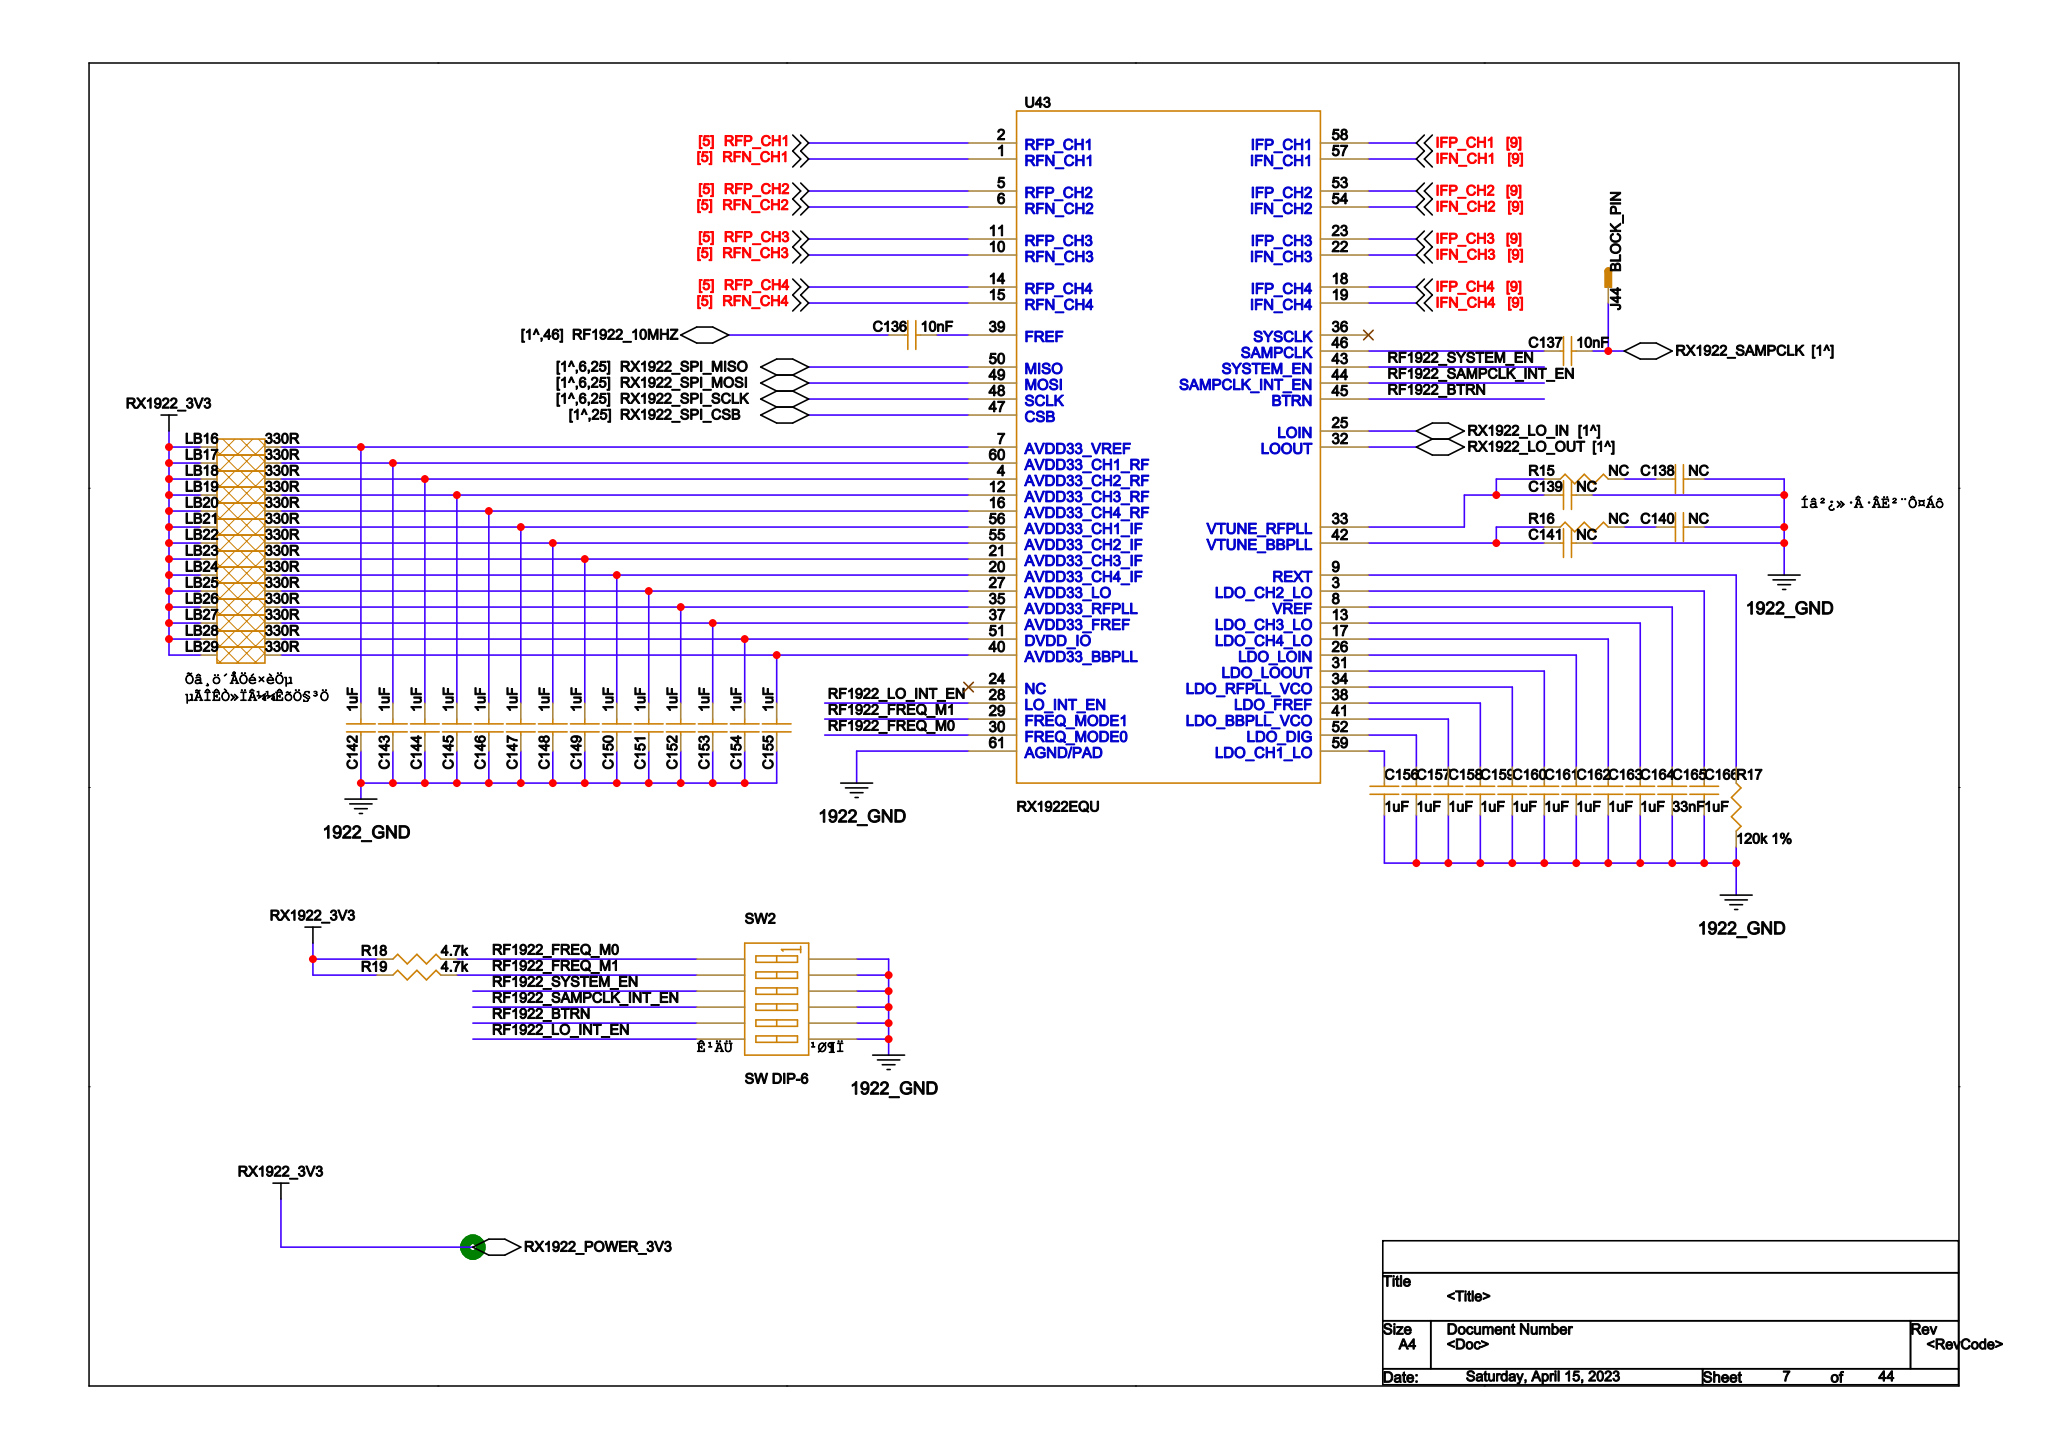Circuit board | Cadence Allegro | 1034 parts | 912 nets | one sheet of the schematic
Parts on this sheet (reference | value | footprint):
C136 | 10nF | C0402
C137 | 10nF | C0402
C138 | NC | C0402
C139 | NC | C0402
C140 | NC | C0402
C141 | NC | C0402
C142 | 1uF | C0402
C143 | 1uF | C0402
C144 | 1uF | C0402
C145 | 1uF | C0402
C146 | 1uF | C0402
C147 | 1uF | C0402
C148 | 1uF | C0402
C149 | 1uF | C0402
C150 | 1uF | C0402
C151 | 1uF | C0402
C152 | 1uF | C0402
C153 | 1uF | C0402
C154 | 1uF | C0402
C155 | 1uF | C0402
C156 | 1uF | C0402
C157 | 1uF | C0402
C158 | 1uF | C0402
C159 | 1uF | C0402
C160 | 1uF | C0402
C161 | 1uF | C0402
C162 | 1uF | C0402
C163 | 1uF | C0402
C164 | 1uF | C0402
C165 | 33nF | C0402
C166 | 1uF | C0402
J44 | BLOCK_PIN | B_PIN_SMD
LB16 | 330R | LB0402
LB17 | 330R | LB0402
LB18 | 330R | LB0402
LB19 | 330R | LB0402
LB20 | 330R | LB0402
LB21 | 330R | LB0402
LB22 | 330R | LB0402
LB23 | 330R | LB0402
LB24 | 330R | LB0402
LB25 | 330R | LB0402
LB26 | 330R | LB0402
LB27 | 330R | LB0402
LB28 | 330R | LB0402
LB29 | 330R | LB0402
R15 | NC | R0402
R16 | NC | R0402
R17 | 120k 1% | R0402
R18 | 4.7k | R0402
R19 | 4.7k | R0402
SW2 | SW DIP-6 | SW_6_SOP
U43 | RX1922EQU | RX1922_QFN60
Nets of these parts (net: part-pin ...):
N188074: C137-2 J44-1
1922_GND: C138-2 C139-2 C140-2 C141-2 C142-1 C143-1 C144-1 C145-1 C146-1 C147-1 C148-1 C149-1 C150-1 C151-1 C152-1 C153-1 C154-1 C155-1 C156-2 C157-2 C158-2 C159-2 C160-2 C161-2 C162-2 C163-2 C164-2 C165-2 C166-2 R17-2 SW2-7 SW2-8 SW2-9 SW2-10 SW2-11 SW2-12 U43-61
PWR1922_3V3_2: LB16-1 LB17-1 LB18-1 LB19-1 LB20-1 LB21-1 LB22-1 LB23-1 LB24-1 LB25-1 LB26-1 LB27-1 LB28-1 LB29-1 R18-1 R19-1
N424726_D2: C142-2 LB16-2 U43-7
N424730_D2: C143-2 LB17-2 U43-60
N424678_D2: C144-2 LB18-2 U43-4
N424682_D2: C145-2 LB19-2 U43-12
N424686_D2: C146-2 LB20-2 U43-16
N424690_D2: C147-2 LB21-2 U43-56
N424694_D2: C148-2 LB22-2 U43-55
N424698_D2: C149-2 LB23-2 U43-21
N424630_D2: C150-2 LB24-2 U43-20
N424634_D2: C151-2 LB25-2 U43-27
N424606_D2: C152-2 LB26-2 U43-35
N424610_D2: C153-2 LB27-2 U43-37
N424588_D2: C154-2 LB28-2 U43-51
N424576_D2: C155-2 LB29-2 U43-40
RF1922_10MHZ: C136-1
N426726_D2: C136-2 U43-39
N426273_D2: C137-1 U43-46
N425592_D2: C138-1 R15-2
N425584_D2: C139-1 R15-1 U43-33
N425372_D2: C140-1 R16-2
N425300_D2: C141-1 R16-1 U43-42
N382314_D2: C156-1 U43-59
N382275_D2: C157-1 U43-52
N382268_D2: C158-1 U43-41
N382255_D2: C159-1 U43-38
N382242_D2: C160-1 U43-34
N382235_D2: C161-1 U43-31
N382222_D2: C162-1 U43-26
N382215_D2: C163-1 U43-17
N382202_D2: C164-1 U43-13
N382176_D2: C166-1 U43-3
N382189_D2: C165-1 U43-8
RF1922_FREQ_M0_D2: R18-2 SW2-1 U43-30
RF1922_FREQ_M1_D2: R19-2 SW2-2 U43-29
N382169_D2: R17-1 U43-9
RF1922_SYSTEM_EN_D2: SW2-3 U43-43
RF1922_SAMPCLK_INT_EN_D2: SW2-4 U43-44
RF1922_BTRN_D2: SW2-5 U43-45
RF1922_LO_INT_EN_D2: SW2-6 U43-28
RX1922_LO_OUT: U43-32